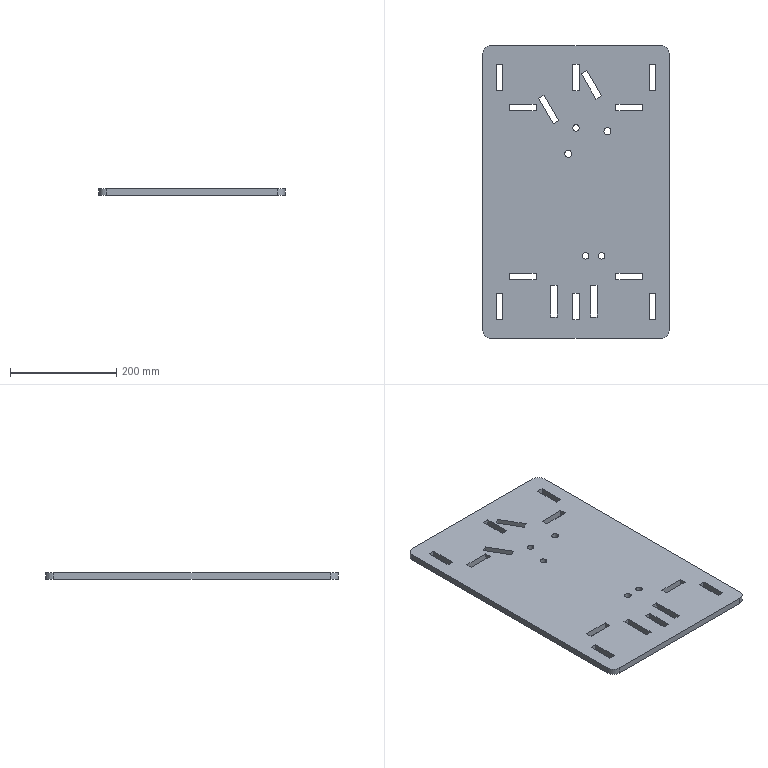Part | SolidWorks | features FlatPattern 1, SMBaseFlange 1, SheetMetal 1 | 1 solid | 76 faces | box 350 x 550 x 12 mm | volume 2194959 mm3 | plane 62 | cylinder 14 | commonest cylinder face diameters 12.5 x6 13 x4 30 x4